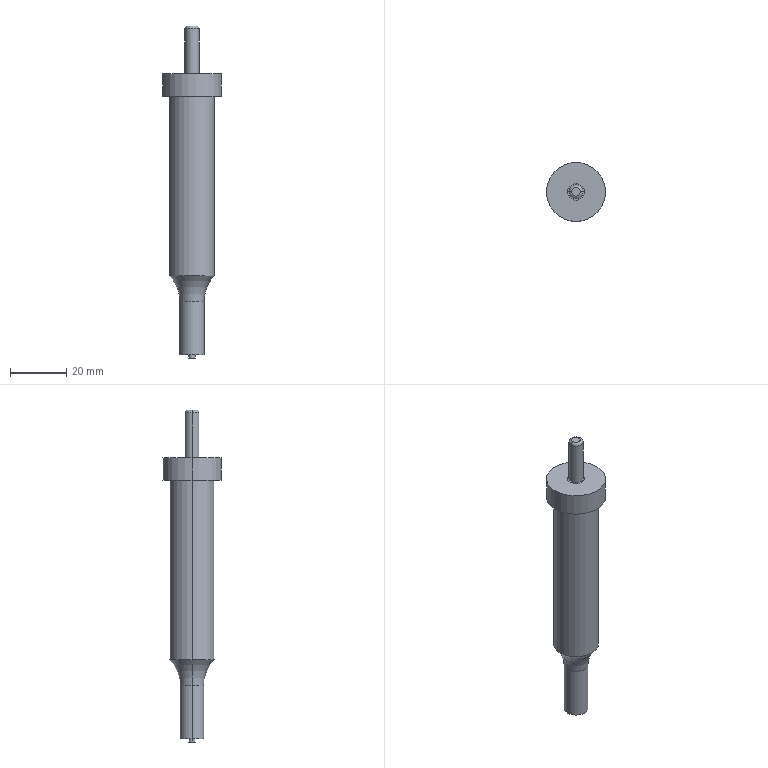Part | STEP file | 1_id282_x_t | 1 solid | 22 faces | box 21 x 21 x 118.2 mm | volume 17923 mm3 | cylinder 12 | plane 6 | torus 4 | commonest cylinder face diameters 2.26 x2 5 x2 6 x2 8.55 x2 16 x2 21 x2
STEP:
#1=CARTESIAN_POINT('',(3701.,59.5,84.5));
#2=VERTEX_POINT('',#1);
#3=CARTESIAN_POINT('',(3701.,59.5,92.5));
#4=VERTEX_POINT('',#3);
#5=CARTESIAN_POINT('',(3701.,59.5,88.5));
#6=DIRECTION('',(0.,0.,1.));
#7=VECTOR('',#6,1.);
#8=LINE('',#5,#7);
#9=EDGE_CURVE('',#2,#4,#8,.T.);
#10=ORIENTED_EDGE('',*,*,#9,.F.);
#11=CARTESIAN_POINT('',(3680.,59.5,84.5));
#12=VERTEX_POINT('',#11);
#13=CARTESIAN_POINT('',(3690.5,59.5,84.5));
#14=DIRECTION('',(0.,0.,1.));
#15=DIRECTION('',(1.,0.,0.));
#16=AXIS2_PLACEMENT_3D('',#13,#14,#15);
#17=CIRCLE('',#16,10.5);
#18=EDGE_CURVE('',#2,#12,#17,.T.);
#19=ORIENTED_EDGE('',*,*,#18,.T.);
#20=CARTESIAN_POINT('',(3680.,59.5,92.5));
#21=VERTEX_POINT('',#20);
#22=CARTESIAN_POINT('',(3680.,59.5,88.5));
#23=DIRECTION('',(0.,0.,-1.));
#24=VECTOR('',#23,1.);
#25=LINE('',#22,#24);
#26=EDGE_CURVE('',#21,#12,#25,.T.);
#27=ORIENTED_EDGE('',*,*,#26,.F.);
#28=CARTESIAN_POINT('',(3690.5,59.5,92.5));
#29=DIRECTION('',(0.,0.,1.));
#30=DIRECTION('',(1.,0.,0.));
#31=AXIS2_PLACEMENT_3D('',#28,#29,#30);
#32=CIRCLE('',#31,10.5);
#33=EDGE_CURVE('',#4,#21,#32,.T.);
#34=ORIENTED_EDGE('',*,*,#33,.F.);
#35=EDGE_LOOP('',(#10,#19,#27,#34));
#36=FACE_OUTER_BOUND('',#35,.T.);
#37=CARTESIAN_POINT('',(3690.5,59.5,88.5));
#38=DIRECTION('',(0.,0.,-1.));
#39=DIRECTION('',(-1.,0.,0.));
#40=AXIS2_PLACEMENT_3D('',#37,#38,#39);
#41=CYLINDRICAL_SURFACE('',#40,10.5);
#42=ADVANCED_FACE('',(#36),#41,.T.);
#43=CARTESIAN_POINT('',(3698.5,59.5,20.609));
#44=VERTEX_POINT('',#43);
#45=CARTESIAN_POINT('',(3698.5,59.5,84.5));
#46=VERTEX_POINT('',#45);
#47=CARTESIAN_POINT('',(3698.5,59.5,38.5));
#48=DIRECTION('',(0.,0.,1.));
#49=VECTOR('',#48,1.);
#50=LINE('',#47,#49);
#51=EDGE_CURVE('',#44,#46,#50,.T.);
#52=ORIENTED_EDGE('',*,*,#51,.F.);
#53=CARTESIAN_POINT('',(3682.5,59.5,20.609));
#54=VERTEX_POINT('',#53);
#55=CARTESIAN_POINT('',(3690.5,59.5,20.609));
#56=DIRECTION('',(0.,0.,1.));
#57=DIRECTION('',(1.,0.,0.));
#58=AXIS2_PLACEMENT_3D('',#55,#56,#57);
#59=CIRCLE('',#58,8.);
#60=EDGE_CURVE('',#44,#54,#59,.T.);
#61=ORIENTED_EDGE('',*,*,#60,.T.);
#62=CARTESIAN_POINT('',(3682.5,59.5,84.5));
#63=VERTEX_POINT('',#62);
#64=CARTESIAN_POINT('',(3682.5,59.5,38.5));
#65=DIRECTION('',(0.,0.,-1.));
#66=VECTOR('',#65,1.);
#67=LINE('',#64,#66);
#68=EDGE_CURVE('',#63,#54,#67,.T.);
#69=ORIENTED_EDGE('',*,*,#68,.F.);
#70=CARTESIAN_POINT('',(3690.5,59.5,84.5));
#71=DIRECTION('',(0.,0.,1.));
#72=DIRECTION('',(1.,0.,0.));
#73=AXIS2_PLACEMENT_3D('',#70,#71,#72);
#74=CIRCLE('',#73,8.);
#75=EDGE_CURVE('',#46,#63,#74,.T.);
#76=ORIENTED_EDGE('',*,*,#75,.F.);
#77=EDGE_LOOP('',(#52,#61,#69,#76));
#78=FACE_OUTER_BOUND('',#77,.T.);
#79=CARTESIAN_POINT('',(3690.5,59.5,38.5));
#80=DIRECTION('',(0.,0.,-1.));
#81=DIRECTION('',(-1.,0.,0.));
#82=AXIS2_PLACEMENT_3D('',#79,#80,#81);
#83=CYLINDRICAL_SURFACE('',#82,8.);
#84=ADVANCED_FACE('',(#78),#83,.T.);
#85=CARTESIAN_POINT('',(3694.775,59.5,11.5));
#86=VERTEX_POINT('',#85);
#87=CARTESIAN_POINT('',(3694.775,59.5,-7.5));
#88=VERTEX_POINT('',#87);
#89=CARTESIAN_POINT('',(3694.775,59.5,2.));
#90=DIRECTION('',(0.,0.,-1.));
#91=VECTOR('',#90,1.);
#92=LINE('',#89,#91);
#93=EDGE_CURVE('',#86,#88,#92,.T.);
#94=ORIENTED_EDGE('',*,*,#93,.F.);
#95=CARTESIAN_POINT('',(3686.225,59.5,11.5));
#96=VERTEX_POINT('',#95);
#97=CARTESIAN_POINT('',(3690.5,59.5,11.5));
#98=DIRECTION('',(0.,0.,1.));
#99=DIRECTION('',(1.,0.,0.));
#100=AXIS2_PLACEMENT_3D('',#97,#98,#99);
#101=CIRCLE('',#100,4.275);
#102=EDGE_CURVE('',#96,#86,#101,.T.);
#103=ORIENTED_EDGE('',*,*,#102,.F.);
#104=CARTESIAN_POINT('',(3686.225,59.5,-7.5));
#105=VERTEX_POINT('',#104);
#106=CARTESIAN_POINT('',(3686.225,59.5,2.));
#107=DIRECTION('',(0.,0.,1.));
#108=VECTOR('',#107,1.);
#109=LINE('',#106,#108);
#110=EDGE_CURVE('',#105,#96,#109,.T.);
#111=ORIENTED_EDGE('',*,*,#110,.F.);
#112=CARTESIAN_POINT('',(3690.5,59.5,-7.5));
#113=DIRECTION('',(0.,0.,-1.));
#114=DIRECTION('',(1.,0.,0.));
#115=AXIS2_PLACEMENT_3D('',#112,#113,#114);
#116=CIRCLE('',#115,4.275);
#117=EDGE_CURVE('',#88,#105,#116,.T.);
#118=ORIENTED_EDGE('',*,*,#117,.F.);
#119=EDGE_LOOP('',(#94,#103,#111,#118));
#120=FACE_OUTER_BOUND('',#119,.T.);
#121=CARTESIAN_POINT('',(3690.5,59.5,2.));
#122=DIRECTION('',(0.,0.,-1.));
#123=DIRECTION('',(-1.,0.,0.));
#124=AXIS2_PLACEMENT_3D('',#121,#122,#123);
#125=CYLINDRICAL_SURFACE('',#124,4.275);
#126=ADVANCED_FACE('',(#120),#125,.T.);
#127=CARTESIAN_POINT('',(3673.225,59.5,11.5));
#128=DIRECTION('',(0.,-1.,0.));
#129=DIRECTION('',(-1.,0.,0.));
#130=AXIS2_PLACEMENT_3D('',#127,#128,#129);
#131=CIRCLE('',#130,13.);
#132=EDGE_CURVE('',#96,#54,#131,.T.);
#133=ORIENTED_EDGE('',*,*,#132,.F.);
#134=ORIENTED_EDGE('',*,*,#102,.T.);
#135=CARTESIAN_POINT('',(3707.775,59.5,11.5));
#136=DIRECTION('',(0.,-1.,0.));
#137=DIRECTION('',(1.,0.,0.));
#138=AXIS2_PLACEMENT_3D('',#135,#136,#137);
#139=CIRCLE('',#138,13.);
#140=EDGE_CURVE('',#44,#86,#139,.T.);
#141=ORIENTED_EDGE('',*,*,#140,.F.);
#142=CARTESIAN_POINT('',(3690.5,59.5,20.609));
#143=DIRECTION('',(0.,0.,1.));
#144=DIRECTION('',(1.,0.,0.));
#145=AXIS2_PLACEMENT_3D('',#142,#143,#144);
#146=CIRCLE('',#145,8.);
#147=EDGE_CURVE('',#54,#44,#146,.T.);
#148=ORIENTED_EDGE('',*,*,#147,.F.);
#149=EDGE_LOOP('',(#133,#134,#141,#148));
#150=FACE_OUTER_BOUND('',#149,.T.);
#151=CARTESIAN_POINT('',(3690.5,59.5,11.5));
#152=DIRECTION('',(0.,0.,1.));
#153=DIRECTION('',(1.,0.,0.));
#154=AXIS2_PLACEMENT_3D('',#151,#152,#153);
#155=TOROIDAL_SURFACE('',#154,17.275,13.);
#156=ADVANCED_FACE('',(#150),#155,.F.);
#157=CARTESIAN_POINT('',(3689.37,59.5,-7.5));
#158=VERTEX_POINT('',#157);
#159=CARTESIAN_POINT('',(3689.37,59.5,-8.7));
#160=VERTEX_POINT('',#159);
#161=CARTESIAN_POINT('',(3689.37,59.5,-7.5));
#162=DIRECTION('',(0.,0.,-1.));
#163=VECTOR('',#162,1.);
#164=LINE('',#161,#163);
#165=EDGE_CURVE('',#158,#160,#164,.T.);
#166=ORIENTED_EDGE('',*,*,#165,.F.);
#167=CARTESIAN_POINT('',(3691.63,59.5,-7.5));
#168=VERTEX_POINT('',#167);
#169=CARTESIAN_POINT('',(3690.5,59.5,-7.5));
#170=DIRECTION('',(0.,0.,1.));
#171=DIRECTION('',(-1.,0.,0.));
#172=AXIS2_PLACEMENT_3D('',#169,#170,#171);
#173=CIRCLE('',#172,1.13);
#174=EDGE_CURVE('',#168,#158,#173,.T.);
#175=ORIENTED_EDGE('',*,*,#174,.F.);
#176=CARTESIAN_POINT('',(3691.63,59.5,-8.7));
#177=VERTEX_POINT('',#176);
#178=CARTESIAN_POINT('',(3691.63,59.5,-7.5));
#179=DIRECTION('',(0.,0.,1.));
#180=VECTOR('',#179,1.);
#181=LINE('',#178,#180);
#182=EDGE_CURVE('',#177,#168,#181,.T.);
#183=ORIENTED_EDGE('',*,*,#182,.F.);
#184=CARTESIAN_POINT('',(3690.5,59.5,-8.7));
#185=DIRECTION('',(0.,0.,1.));
#186=DIRECTION('',(-1.,0.,0.));
#187=AXIS2_PLACEMENT_3D('',#184,#185,#186);
#188=CIRCLE('',#187,1.13);
#189=EDGE_CURVE('',#177,#160,#188,.T.);
#190=ORIENTED_EDGE('',*,*,#189,.T.);
#191=EDGE_LOOP('',(#166,#175,#183,#190));
#192=FACE_OUTER_BOUND('',#191,.T.);
#193=CARTESIAN_POINT('',(3690.5,59.5,-7.5));
#194=DIRECTION('',(0.,0.,1.));
#195=DIRECTION('',(1.,0.,0.));
#196=AXIS2_PLACEMENT_3D('',#193,#194,#195);
#197=CYLINDRICAL_SURFACE('',#196,1.13);
#198=ADVANCED_FACE('',(#192),#197,.T.);
#199=CARTESIAN_POINT('',(3688.,59.5,108.5));
#200=VERTEX_POINT('',#199);
#201=CARTESIAN_POINT('',(3688.,59.5,92.6));
#202=VERTEX_POINT('',#201);
#203=CARTESIAN_POINT('',(3688.,59.5,100.55));
#204=DIRECTION('',(0.,0.,-1.));
#205=VECTOR('',#204,1.);
#206=LINE('',#203,#205);
#207=EDGE_CURVE('',#200,#202,#206,.T.);
#208=ORIENTED_EDGE('',*,*,#207,.F.);
#209=CARTESIAN_POINT('',(3693.,59.5,108.5));
#210=VERTEX_POINT('',#209);
#211=CARTESIAN_POINT('',(3690.5,59.5,108.5));
#212=DIRECTION('',(0.,0.,-1.));
#213=DIRECTION('',(-1.,0.,0.));
#214=AXIS2_PLACEMENT_3D('',#211,#212,#213);
#215=CIRCLE('',#214,2.5);
#216=EDGE_CURVE('',#200,#210,#215,.T.);
#217=ORIENTED_EDGE('',*,*,#216,.T.);
#218=CARTESIAN_POINT('',(3693.,59.5,92.6));
#219=VERTEX_POINT('',#218);
#220=CARTESIAN_POINT('',(3693.,59.5,100.55));
#221=DIRECTION('',(0.,0.,1.));
#222=VECTOR('',#221,1.);
#223=LINE('',#220,#222);
#224=EDGE_CURVE('',#219,#210,#223,.T.);
#225=ORIENTED_EDGE('',*,*,#224,.F.);
#226=CARTESIAN_POINT('',(3690.5,59.5,92.6));
#227=DIRECTION('',(0.,0.,-1.));
#228=DIRECTION('',(-1.,0.,0.));
#229=AXIS2_PLACEMENT_3D('',#226,#227,#228);
#230=CIRCLE('',#229,2.5);
#231=EDGE_CURVE('',#202,#219,#230,.T.);
#232=ORIENTED_EDGE('',*,*,#231,.F.);
#233=EDGE_LOOP('',(#208,#217,#225,#232));
#234=FACE_OUTER_BOUND('',#233,.T.);
#235=CARTESIAN_POINT('',(3690.5,59.5,100.55));
#236=DIRECTION('',(0.,0.,1.));
#237=DIRECTION('',(1.,0.,0.));
#238=AXIS2_PLACEMENT_3D('',#235,#236,#237);
#239=CYLINDRICAL_SURFACE('',#238,2.5);
#240=ADVANCED_FACE('',(#234),#239,.T.);
#241=CARTESIAN_POINT('',(3692.,59.5,109.5));
#242=VERTEX_POINT('',#241);
#243=CARTESIAN_POINT('',(3692.,59.5,108.5));
#244=DIRECTION('',(0.,1.,0.));
#245=DIRECTION('',(1.,0.,0.));
#246=AXIS2_PLACEMENT_3D('',#243,#244,#245);
#247=CIRCLE('',#246,1.);
#248=EDGE_CURVE('',#242,#210,#247,.T.);
#249=ORIENTED_EDGE('',*,*,#248,.F.);
#250=CARTESIAN_POINT('',(3689.,59.5,109.5));
#251=VERTEX_POINT('',#250);
#252=CARTESIAN_POINT('',(3690.5,59.5,109.5));
#253=DIRECTION('',(0.,0.,-1.));
#254=DIRECTION('',(-1.,0.,0.));
#255=AXIS2_PLACEMENT_3D('',#252,#253,#254);
#256=CIRCLE('',#255,1.5);
#257=EDGE_CURVE('',#242,#251,#256,.T.);
#258=ORIENTED_EDGE('',*,*,#257,.T.);
#259=CARTESIAN_POINT('',(3689.,59.5,108.5));
#260=DIRECTION('',(0.,1.,0.));
#261=DIRECTION('',(-1.,0.,0.));
#262=AXIS2_PLACEMENT_3D('',#259,#260,#261);
#263=CIRCLE('',#262,1.);
#264=EDGE_CURVE('',#200,#251,#263,.T.);
#265=ORIENTED_EDGE('',*,*,#264,.F.);
#266=CARTESIAN_POINT('',(3690.5,59.5,108.5));
#267=DIRECTION('',(0.,0.,-1.));
#268=DIRECTION('',(-1.,0.,0.));
#269=AXIS2_PLACEMENT_3D('',#266,#267,#268);
#270=CIRCLE('',#269,2.5);
#271=EDGE_CURVE('',#210,#200,#270,.T.);
#272=ORIENTED_EDGE('',*,*,#271,.F.);
#273=EDGE_LOOP('',(#249,#258,#265,#272));
#274=FACE_OUTER_BOUND('',#273,.T.);
#275=CARTESIAN_POINT('',(3690.5,59.5,108.5));
#276=DIRECTION('',(0.,0.,-1.));
#277=DIRECTION('',(-1.,0.,0.));
#278=AXIS2_PLACEMENT_3D('',#275,#276,#277);
#279=TOROIDAL_SURFACE('',#278,1.5,1.);
#280=ADVANCED_FACE('',(#274),#279,.T.);
#281=CARTESIAN_POINT('',(3687.5,59.5,92.6));
#282=VERTEX_POINT('',#281);
#283=CARTESIAN_POINT('',(3687.5,59.5,92.5));
#284=VERTEX_POINT('',#283);
#285=CARTESIAN_POINT('',(3687.5,59.5,92.55));
#286=DIRECTION('',(0.,0.,-1.));
#287=VECTOR('',#286,1.);
#288=LINE('',#285,#287);
#289=EDGE_CURVE('',#282,#284,#288,.T.);
#290=ORIENTED_EDGE('',*,*,#289,.F.);
#291=CARTESIAN_POINT('',(3693.5,59.5,92.6));
#292=VERTEX_POINT('',#291);
#293=CARTESIAN_POINT('',(3690.5,59.5,92.6));
#294=DIRECTION('',(0.,0.,-1.));
#295=DIRECTION('',(-1.,0.,0.));
#296=AXIS2_PLACEMENT_3D('',#293,#294,#295);
#297=CIRCLE('',#296,3.);
#298=EDGE_CURVE('',#282,#292,#297,.T.);
#299=ORIENTED_EDGE('',*,*,#298,.T.);
#300=CARTESIAN_POINT('',(3693.5,59.5,92.5));
#301=VERTEX_POINT('',#300);
#302=CARTESIAN_POINT('',(3693.5,59.5,92.55));
#303=DIRECTION('',(0.,0.,1.));
#304=VECTOR('',#303,1.);
#305=LINE('',#302,#304);
#306=EDGE_CURVE('',#301,#292,#305,.T.);
#307=ORIENTED_EDGE('',*,*,#306,.F.);
#308=CARTESIAN_POINT('',(3690.5,59.5,92.5));
#309=DIRECTION('',(0.,0.,-1.));
#310=DIRECTION('',(-1.,0.,0.));
#311=AXIS2_PLACEMENT_3D('',#308,#309,#310);
#312=CIRCLE('',#311,3.);
#313=EDGE_CURVE('',#284,#301,#312,.T.);
#314=ORIENTED_EDGE('',*,*,#313,.F.);
#315=EDGE_LOOP('',(#290,#299,#307,#314));
#316=FACE_OUTER_BOUND('',#315,.T.);
#317=CARTESIAN_POINT('',(3690.5,59.5,87.05));
#318=DIRECTION('',(0.,0.,1.));
#319=DIRECTION('',(1.,0.,0.));
#320=AXIS2_PLACEMENT_3D('',#317,#318,#319);
#321=CYLINDRICAL_SURFACE('',#320,3.);
#322=ADVANCED_FACE('',(#316),#321,.T.);
#323=ORIENTED_EDGE('',*,*,#289,.T.);
#324=CARTESIAN_POINT('',(3690.5,59.5,92.5));
#325=DIRECTION('',(0.,0.,-1.));
#326=DIRECTION('',(-1.,0.,0.));
#327=AXIS2_PLACEMENT_3D('',#324,#325,#326);
#328=CIRCLE('',#327,3.);
#329=EDGE_CURVE('',#301,#284,#328,.T.);
#330=ORIENTED_EDGE('',*,*,#329,.F.);
#331=ORIENTED_EDGE('',*,*,#306,.T.);
#332=CARTESIAN_POINT('',(3690.5,59.5,92.6));
#333=DIRECTION('',(0.,0.,-1.));
#334=DIRECTION('',(-1.,0.,0.));
#335=AXIS2_PLACEMENT_3D('',#332,#333,#334);
#336=CIRCLE('',#335,3.);
#337=EDGE_CURVE('',#292,#282,#336,.T.);
#338=ORIENTED_EDGE('',*,*,#337,.T.);
#339=EDGE_LOOP('',(#323,#330,#331,#338));
#340=FACE_OUTER_BOUND('',#339,.T.);
#341=CARTESIAN_POINT('',(3690.5,59.5,87.05));
#342=DIRECTION('',(0.,0.,1.));
#343=DIRECTION('',(1.,0.,0.));
#344=AXIS2_PLACEMENT_3D('',#341,#342,#343);
#345=CYLINDRICAL_SURFACE('',#344,3.);
#346=ADVANCED_FACE('',(#340),#345,.T.);
#347=CARTESIAN_POINT('',(3690.5,59.5,109.5));
#348=DIRECTION('',(0.,0.,-1.));
#349=DIRECTION('',(-1.,0.,0.));
#350=AXIS2_PLACEMENT_3D('',#347,#348,#349);
#351=CIRCLE('',#350,1.5);
#352=EDGE_CURVE('',#251,#242,#351,.T.);
#353=ORIENTED_EDGE('',*,*,#352,.F.);
#354=ORIENTED_EDGE('',*,*,#257,.F.);
#355=EDGE_LOOP('',(#353,#354));
#356=FACE_OUTER_BOUND('',#355,.T.);
#357=CARTESIAN_POINT('',(3689.75,59.5,109.5));
#358=DIRECTION('',(0.,0.,1.));
#359=DIRECTION('',(-1.,0.,0.));
#360=AXIS2_PLACEMENT_3D('',#357,#358,#359);
#361=PLANE('',#360);
#362=ADVANCED_FACE('',(#356),#361,.T.);
#363=ORIENTED_EDGE('',*,*,#248,.T.);
#364=ORIENTED_EDGE('',*,*,#216,.F.);
#365=ORIENTED_EDGE('',*,*,#264,.T.);
#366=ORIENTED_EDGE('',*,*,#352,.T.);
#367=EDGE_LOOP('',(#363,#364,#365,#366));
#368=FACE_OUTER_BOUND('',#367,.T.);
#369=CARTESIAN_POINT('',(3690.5,59.5,108.5));
#370=DIRECTION('',(0.,0.,-1.));
#371=DIRECTION('',(-1.,0.,0.));
#372=AXIS2_PLACEMENT_3D('',#369,#370,#371);
#373=TOROIDAL_SURFACE('',#372,1.5,1.);
#374=ADVANCED_FACE('',(#368),#373,.T.);
#375=ORIENTED_EDGE('',*,*,#207,.T.);
#376=CARTESIAN_POINT('',(3690.5,59.5,92.6));
#377=DIRECTION('',(0.,0.,-1.));
#378=DIRECTION('',(-1.,0.,0.));
#379=AXIS2_PLACEMENT_3D('',#376,#377,#378);
#380=CIRCLE('',#379,2.5);
#381=EDGE_CURVE('',#219,#202,#380,.T.);
#382=ORIENTED_EDGE('',*,*,#381,.F.);
#383=ORIENTED_EDGE('',*,*,#224,.T.);
#384=ORIENTED_EDGE('',*,*,#271,.T.);
#385=EDGE_LOOP('',(#375,#382,#383,#384));
#386=FACE_OUTER_BOUND('',#385,.T.);
#387=CARTESIAN_POINT('',(3690.5,59.5,100.55));
#388=DIRECTION('',(0.,0.,1.));
#389=DIRECTION('',(1.,0.,0.));
#390=AXIS2_PLACEMENT_3D('',#387,#388,#389);
#391=CYLINDRICAL_SURFACE('',#390,2.5);
#392=ADVANCED_FACE('',(#386),#391,.T.);
#393=ORIENTED_EDGE('',*,*,#298,.F.);
#394=ORIENTED_EDGE('',*,*,#337,.F.);
#395=EDGE_LOOP('',(#393,#394));
#396=FACE_BOUND('',#395,.T.);
#397=ORIENTED_EDGE('',*,*,#231,.T.);
#398=ORIENTED_EDGE('',*,*,#381,.T.);
#399=EDGE_LOOP('',(#397,#398));
#400=FACE_BOUND('',#399,.T.);
#401=CARTESIAN_POINT('',(3687.75,59.5,92.6));
#402=DIRECTION('',(0.,0.,1.));
#403=DIRECTION('',(-1.,0.,0.));
#404=AXIS2_PLACEMENT_3D('',#401,#402,#403);
#405=PLANE('',#404);
#406=ADVANCED_FACE('',(#396,#400),#405,.T.);
#407=ORIENTED_EDGE('',*,*,#165,.T.);
#408=CARTESIAN_POINT('',(3690.5,59.5,-8.7));
#409=DIRECTION('',(0.,0.,1.));
#410=DIRECTION('',(-1.,0.,0.));
#411=AXIS2_PLACEMENT_3D('',#408,#409,#410);
#412=CIRCLE('',#411,1.13);
#413=EDGE_CURVE('',#160,#177,#412,.T.);
#414=ORIENTED_EDGE('',*,*,#413,.T.);
#415=ORIENTED_EDGE('',*,*,#182,.T.);
#416=CARTESIAN_POINT('',(3690.5,59.5,-7.5));
#417=DIRECTION('',(0.,0.,1.));
#418=DIRECTION('',(-1.,0.,0.));
#419=AXIS2_PLACEMENT_3D('',#416,#417,#418);
#420=CIRCLE('',#419,1.13);
#421=EDGE_CURVE('',#158,#168,#420,.T.);
#422=ORIENTED_EDGE('',*,*,#421,.F.);
#423=EDGE_LOOP('',(#407,#414,#415,#422));
#424=FACE_OUTER_BOUND('',#423,.T.);
#425=CARTESIAN_POINT('',(3690.5,59.5,-7.5));
#426=DIRECTION('',(0.,0.,1.));
#427=DIRECTION('',(1.,0.,0.));
#428=AXIS2_PLACEMENT_3D('',#425,#426,#427);
#429=CYLINDRICAL_SURFACE('',#428,1.13);
#430=ADVANCED_FACE('',(#424),#429,.T.);
#431=ORIENTED_EDGE('',*,*,#413,.F.);
#432=ORIENTED_EDGE('',*,*,#189,.F.);
#433=EDGE_LOOP('',(#431,#432));
#434=FACE_OUTER_BOUND('',#433,.T.);
#435=CARTESIAN_POINT('',(3690.5,59.5,-8.7));
#436=DIRECTION('',(0.,0.,1.));
#437=DIRECTION('',(1.,0.,0.));
#438=AXIS2_PLACEMENT_3D('',#435,#436,#437);
#439=PLANE('',#438);
#440=ADVANCED_FACE('',(#434),#439,.F.);
#441=ORIENTED_EDGE('',*,*,#132,.T.);
#442=ORIENTED_EDGE('',*,*,#60,.F.);
#443=ORIENTED_EDGE('',*,*,#140,.T.);
#444=CARTESIAN_POINT('',(3690.5,59.5,11.5));
#445=DIRECTION('',(0.,0.,1.));
#446=DIRECTION('',(1.,0.,0.));
#447=AXIS2_PLACEMENT_3D('',#444,#445,#446);
#448=CIRCLE('',#447,4.275);
#449=EDGE_CURVE('',#86,#96,#448,.T.);
#450=ORIENTED_EDGE('',*,*,#449,.T.);
#451=EDGE_LOOP('',(#441,#442,#443,#450));
#452=FACE_OUTER_BOUND('',#451,.T.);
#453=CARTESIAN_POINT('',(3690.5,59.5,11.5));
#454=DIRECTION('',(0.,0.,1.));
#455=DIRECTION('',(1.,0.,0.));
#456=AXIS2_PLACEMENT_3D('',#453,#454,#455);
#457=TOROIDAL_SURFACE('',#456,17.275,13.);
#458=ADVANCED_FACE('',(#452),#457,.F.);
#459=ORIENTED_EDGE('',*,*,#93,.T.);
#460=CARTESIAN_POINT('',(3690.5,59.5,-7.5));
#461=DIRECTION('',(0.,0.,-1.));
#462=DIRECTION('',(1.,0.,0.));
#463=AXIS2_PLACEMENT_3D('',#460,#461,#462);
#464=CIRCLE('',#463,4.275);
#465=EDGE_CURVE('',#105,#88,#464,.T.);
#466=ORIENTED_EDGE('',*,*,#465,.F.);
#467=ORIENTED_EDGE('',*,*,#110,.T.);
#468=ORIENTED_EDGE('',*,*,#449,.F.);
#469=EDGE_LOOP('',(#459,#466,#467,#468));
#470=FACE_OUTER_BOUND('',#469,.T.);
#471=CARTESIAN_POINT('',(3690.5,59.5,2.));
#472=DIRECTION('',(0.,0.,-1.));
#473=DIRECTION('',(-1.,0.,0.));
#474=AXIS2_PLACEMENT_3D('',#471,#472,#473);
#475=CYLINDRICAL_SURFACE('',#474,4.275);
#476=ADVANCED_FACE('',(#470),#475,.T.);
#477=ORIENTED_EDGE('',*,*,#421,.T.);
#478=ORIENTED_EDGE('',*,*,#174,.T.);
#479=EDGE_LOOP('',(#477,#478));
#480=FACE_BOUND('',#479,.T.);
#481=ORIENTED_EDGE('',*,*,#117,.T.);
#482=ORIENTED_EDGE('',*,*,#465,.T.);
#483=EDGE_LOOP('',(#481,#482));
#484=FACE_BOUND('',#483,.T.);
#485=CARTESIAN_POINT('',(3694.5,59.5,-7.5));
#486=DIRECTION('',(0.,0.,-1.));
#487=DIRECTION('',(1.,0.,0.));
#488=AXIS2_PLACEMENT_3D('',#485,#486,#487);
#489=PLANE('',#488);
#490=ADVANCED_FACE('',(#480,#484),#489,.T.);
#491=ORIENTED_EDGE('',*,*,#51,.T.);
#492=CARTESIAN_POINT('',(3690.5,59.5,84.5));
#493=DIRECTION('',(0.,0.,1.));
#494=DIRECTION('',(1.,0.,0.));
#495=AXIS2_PLACEMENT_3D('',#492,#493,#494);
#496=CIRCLE('',#495,8.);
#497=EDGE_CURVE('',#63,#46,#496,.T.);
#498=ORIENTED_EDGE('',*,*,#497,.F.);
#499=ORIENTED_EDGE('',*,*,#68,.T.);
#500=ORIENTED_EDGE('',*,*,#147,.T.);
#501=EDGE_LOOP('',(#491,#498,#499,#500));
#502=FACE_OUTER_BOUND('',#501,.T.);
#503=CARTESIAN_POINT('',(3690.5,59.5,38.5));
#504=DIRECTION('',(0.,0.,-1.));
#505=DIRECTION('',(-1.,0.,0.));
#506=AXIS2_PLACEMENT_3D('',#503,#504,#505);
#507=CYLINDRICAL_SURFACE('',#506,8.);
#508=ADVANCED_FACE('',(#502),#507,.T.);
#509=ORIENTED_EDGE('',*,*,#18,.F.);
#510=CARTESIAN_POINT('',(3690.5,59.5,84.5));
#511=DIRECTION('',(0.,0.,1.));
#512=DIRECTION('',(1.,0.,0.));
#513=AXIS2_PLACEMENT_3D('',#510,#511,#512);
#514=CIRCLE('',#513,10.5);
#515=EDGE_CURVE('',#12,#2,#514,.T.);
#516=ORIENTED_EDGE('',*,*,#515,.F.);
#517=EDGE_LOOP('',(#509,#516));
#518=FACE_BOUND('',#517,.T.);
#519=ORIENTED_EDGE('',*,*,#75,.T.);
#520=ORIENTED_EDGE('',*,*,#497,.T.);
#521=EDGE_LOOP('',(#519,#520));
#522=FACE_BOUND('',#521,.T.);
#523=CARTESIAN_POINT('',(3699.75,59.5,84.5));
#524=DIRECTION('',(0.,0.,-1.));
#525=DIRECTION('',(1.,0.,0.));
#526=AXIS2_PLACEMENT_3D('',#523,#524,#525);
#527=PLANE('',#526);
#528=ADVANCED_FACE('',(#518,#522),#527,.T.);
#529=ORIENTED_EDGE('',*,*,#9,.T.);
#530=CARTESIAN_POINT('',(3690.5,59.5,92.5));
#531=DIRECTION('',(0.,0.,1.));
#532=DIRECTION('',(1.,0.,0.));
#533=AXIS2_PLACEMENT_3D('',#530,#531,#532);
#534=CIRCLE('',#533,10.5);
#535=EDGE_CURVE('',#21,#4,#534,.T.);
#536=ORIENTED_EDGE('',*,*,#535,.F.);
#537=ORIENTED_EDGE('',*,*,#26,.T.);
#538=ORIENTED_EDGE('',*,*,#515,.T.);
#539=EDGE_LOOP('',(#529,#536,#537,#538));
#540=FACE_OUTER_BOUND('',#539,.T.);
#541=CARTESIAN_POINT('',(3690.5,59.5,88.5));
#542=DIRECTION('',(0.,0.,-1.));
#543=DIRECTION('',(-1.,0.,0.));
#544=AXIS2_PLACEMENT_3D('',#541,#542,#543);
#545=CYLINDRICAL_SURFACE('',#544,10.5);
#546=ADVANCED_FACE('',(#540),#545,.T.);
#547=ORIENTED_EDGE('',*,*,#329,.T.);
#548=ORIENTED_EDGE('',*,*,#313,.T.);
#549=EDGE_LOOP('',(#547,#548));
#550=FACE_BOUND('',#549,.T.);
#551=ORIENTED_EDGE('',*,*,#33,.T.);
#552=ORIENTED_EDGE('',*,*,#535,.T.);
#553=EDGE_LOOP('',(#551,#552));
#554=FACE_BOUND('',#553,.T.);
#555=CARTESIAN_POINT('',(3695.75,59.5,92.5));
#556=DIRECTION('',(0.,0.,1.));
#557=DIRECTION('',(-1.,0.,0.));
#558=AXIS2_PLACEMENT_3D('',#555,#556,#557);
#559=PLANE('',#558);
#560=ADVANCED_FACE('',(#550,#554),#559,.T.);
#561=CLOSED_SHELL('',(#42,#84,#126,#156,#198,#240,#280,#322,#346,#362,#374,#392,#406,#430,#440,#458,#476,#490,#508,#528,#546,#560));
#562=MANIFOLD_SOLID_BREP('',#561);
#563=(LENGTH_UNIT()NAMED_UNIT(*)SI_UNIT(.MILLI.,.METRE.));
#564=UNCERTAINTY_MEASURE_WITH_UNIT(LENGTH_MEASURE(0.00002),#563,'','');
#565=(NAMED_UNIT(*)PLANE_ANGLE_UNIT()SI_UNIT($,.RADIAN.));
#566=PLANE_ANGLE_MEASURE_WITH_UNIT(PLANE_ANGLE_MEASURE(0.01745),#565);
#567=DIMENSIONAL_EXPONENTS(0.,0.,0.,0.,0.,0.,0.);
#568=(CONVERSION_BASED_UNIT('DEGREE',#566)NAMED_UNIT(#567)PLANE_ANGLE_UNIT());
#569=(NAMED_UNIT(*)SI_UNIT($,.STERADIAN.)SOLID_ANGLE_UNIT());
#570=(GEOMETRIC_REPRESENTATION_CONTEXT(3)GLOBAL_UNCERTAINTY_ASSIGNED_CONTEXT((#564))GLOBAL_UNIT_ASSIGNED_CONTEXT((#563,#568,#569))REPRESENTATION_CONTEXT('',''));
#571=ADVANCED_BREP_SHAPE_REPRESENTATION('',(#562),#570);